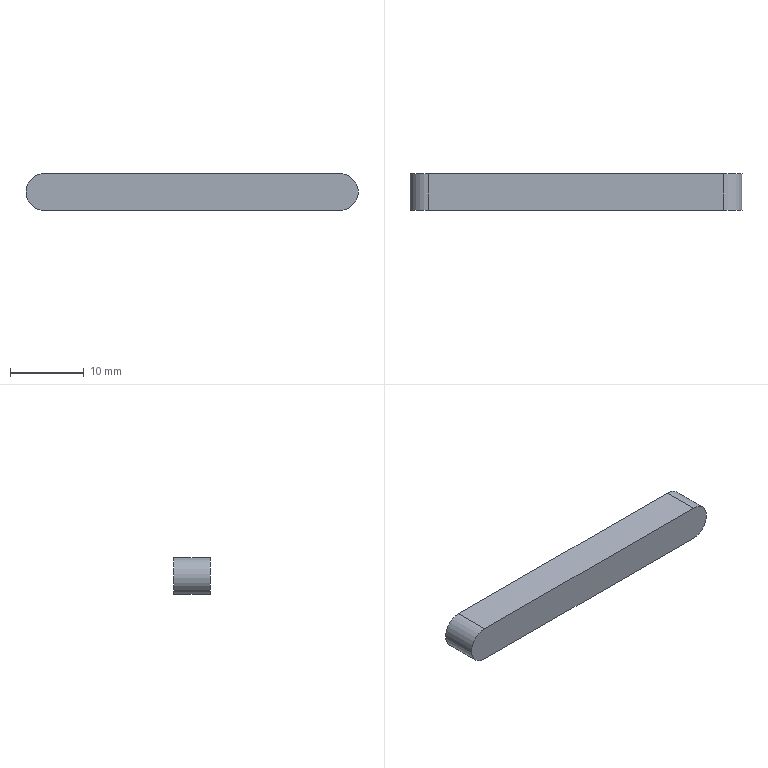Part | STEP file | PN_0046 (5x5x40) | 1 solid | 6 faces | box 45 x 5 x 5 mm | volume 1098 mm3 | plane 4 | cylinder 2 | commonest cylinder face diameters 5 x2
STEP:
#1=CARTESIAN_POINT('',(0.,0.,0.));
#2=DIRECTION('',(0.,0.,1.));
#3=DIRECTION('',(1.,0.,0.));
#4=AXIS2_PLACEMENT_3D('',#1,#2,#3);
#5=CARTESIAN_POINT('',(-20.,0.,-2.5));
#6=VERTEX_POINT('',#5);
#7=CARTESIAN_POINT('',(-20.,0.,2.5));
#8=VERTEX_POINT('',#7);
#9=CARTESIAN_POINT('',(-20.,0.,0.));
#10=DIRECTION('',(0.,1.,0.));
#11=DIRECTION('',(0.,0.,1.));
#12=AXIS2_PLACEMENT_3D('',#9,#10,#11);
#13=CIRCLE('',#12,2.5);
#14=CARTESIAN_POINT('',(-20.,5.,0.));
#15=DIRECTION('',(0.,-1.,0.));
#16=DIRECTION('',(0.,0.,-1.));
#17=AXIS2_PLACEMENT_3D('',#14,#15,#16);
#18=CYLINDRICAL_SURFACE('',#17,2.5);
#19=CARTESIAN_POINT('',(9.425,5.));
#20=DIRECTION('',(-1.,0.));
#21=VECTOR('',#20,1.);
#22=LINE('',#19,#21);
#23=(GEOMETRIC_REPRESENTATION_CONTEXT(2)PARAMETRIC_REPRESENTATION_CONTEXT()REPRESENTATION_CONTEXT('',''));
#24=DEFINITIONAL_REPRESENTATION('',(#22),#23);
#25=PCURVE('',#18,#24);
#26=CARTESIAN_POINT('',(-20.,0.,0.));
#27=DIRECTION('',(0.,1.,0.));
#28=DIRECTION('',(0.,0.,1.));
#29=AXIS2_PLACEMENT_3D('',#26,#27,#28);
#30=PLANE('',#29);
#31=CARTESIAN_POINT('',(0.,0.));
#32=DIRECTION('',(1.,0.));
#33=AXIS2_PLACEMENT_2D('',#31,#32);
#34=CIRCLE('',#33,2.5);
#35=(GEOMETRIC_REPRESENTATION_CONTEXT(2)PARAMETRIC_REPRESENTATION_CONTEXT()REPRESENTATION_CONTEXT('',''));
#36=DEFINITIONAL_REPRESENTATION('',(#34),#35);
#37=PCURVE('',#30,#36);
#38=SURFACE_CURVE('',#13,(#25,#37),.PCURVE_S1.);
#39=EDGE_CURVE('',#6,#8,#38,.T.);
#40=ORIENTED_EDGE('',*,*,#39,.T.);
#41=CARTESIAN_POINT('',(-20.,5.,2.5));
#42=VERTEX_POINT('',#41);
#43=CARTESIAN_POINT('',(-20.,5.,2.5));
#44=DIRECTION('',(0.,-1.,0.));
#45=VECTOR('',#44,1.);
#46=LINE('',#43,#45);
#47=CARTESIAN_POINT('',(3.142,0.));
#48=DIRECTION('',(0.,1.));
#49=VECTOR('',#48,1.);
#50=LINE('',#47,#49);
#51=(GEOMETRIC_REPRESENTATION_CONTEXT(2)PARAMETRIC_REPRESENTATION_CONTEXT()REPRESENTATION_CONTEXT('',''));
#52=DEFINITIONAL_REPRESENTATION('',(#50),#51);
#53=PCURVE('',#18,#52);
#54=CARTESIAN_POINT('',(-20.,5.,2.5));
#55=DIRECTION('',(0.,0.,-1.));
#56=DIRECTION('',(-1.,0.,0.));
#57=AXIS2_PLACEMENT_3D('',#54,#55,#56);
#58=PLANE('',#57);
#59=CARTESIAN_POINT('',(0.,0.));
#60=DIRECTION('',(0.,-1.));
#61=VECTOR('',#60,1.);
#62=LINE('',#59,#61);
#63=(GEOMETRIC_REPRESENTATION_CONTEXT(2)PARAMETRIC_REPRESENTATION_CONTEXT()REPRESENTATION_CONTEXT('',''));
#64=DEFINITIONAL_REPRESENTATION('',(#62),#63);
#65=PCURVE('',#58,#64);
#66=SURFACE_CURVE('',#46,(#53,#65),.PCURVE_S1.);
#67=EDGE_CURVE('',#42,#8,#66,.T.);
#68=ORIENTED_EDGE('',*,*,#67,.F.);
#69=CARTESIAN_POINT('',(-20.,5.,-2.5));
#70=VERTEX_POINT('',#69);
#71=CARTESIAN_POINT('',(-20.,5.,0.));
#72=DIRECTION('',(0.,1.,0.));
#73=DIRECTION('',(0.,0.,1.));
#74=AXIS2_PLACEMENT_3D('',#71,#72,#73);
#75=CIRCLE('',#74,2.5);
#76=CARTESIAN_POINT('',(9.425,0.));
#77=DIRECTION('',(-1.,0.));
#78=VECTOR('',#77,1.);
#79=LINE('',#76,#78);
#80=(GEOMETRIC_REPRESENTATION_CONTEXT(2)PARAMETRIC_REPRESENTATION_CONTEXT()REPRESENTATION_CONTEXT('',''));
#81=DEFINITIONAL_REPRESENTATION('',(#79),#80);
#82=PCURVE('',#18,#81);
#83=CARTESIAN_POINT('',(-20.,5.,0.));
#84=DIRECTION('',(0.,1.,0.));
#85=DIRECTION('',(0.,0.,1.));
#86=AXIS2_PLACEMENT_3D('',#83,#84,#85);
#87=PLANE('',#86);
#88=CARTESIAN_POINT('',(0.,0.));
#89=DIRECTION('',(1.,0.));
#90=AXIS2_PLACEMENT_2D('',#88,#89);
#91=CIRCLE('',#90,2.5);
#92=(GEOMETRIC_REPRESENTATION_CONTEXT(2)PARAMETRIC_REPRESENTATION_CONTEXT()REPRESENTATION_CONTEXT('',''));
#93=DEFINITIONAL_REPRESENTATION('',(#91),#92);
#94=PCURVE('',#87,#93);
#95=SURFACE_CURVE('',#75,(#82,#94),.PCURVE_S1.);
#96=EDGE_CURVE('',#70,#42,#95,.T.);
#97=ORIENTED_EDGE('',*,*,#96,.F.);
#98=CARTESIAN_POINT('',(-20.,5.,-2.5));
#99=DIRECTION('',(0.,-1.,0.));
#100=VECTOR('',#99,1.);
#101=LINE('',#98,#100);
#102=CARTESIAN_POINT('',(6.283,0.));
#103=DIRECTION('',(0.,1.));
#104=VECTOR('',#103,1.);
#105=LINE('',#102,#104);
#106=(GEOMETRIC_REPRESENTATION_CONTEXT(2)PARAMETRIC_REPRESENTATION_CONTEXT()REPRESENTATION_CONTEXT('',''));
#107=DEFINITIONAL_REPRESENTATION('',(#105),#106);
#108=PCURVE('',#18,#107);
#109=CARTESIAN_POINT('',(-20.,5.,-2.5));
#110=DIRECTION('',(0.,0.,1.));
#111=DIRECTION('',(1.,0.,0.));
#112=AXIS2_PLACEMENT_3D('',#109,#110,#111);
#113=PLANE('',#112);
#114=CARTESIAN_POINT('',(0.,0.));
#115=DIRECTION('',(0.,-1.));
#116=VECTOR('',#115,1.);
#117=LINE('',#114,#116);
#118=(GEOMETRIC_REPRESENTATION_CONTEXT(2)PARAMETRIC_REPRESENTATION_CONTEXT()REPRESENTATION_CONTEXT('',''));
#119=DEFINITIONAL_REPRESENTATION('',(#117),#118);
#120=PCURVE('',#113,#119);
#121=SURFACE_CURVE('',#101,(#108,#120),.PCURVE_S1.);
#122=EDGE_CURVE('',#70,#6,#121,.T.);
#123=ORIENTED_EDGE('',*,*,#122,.T.);
#124=EDGE_LOOP('',(#40,#68,#97,#123));
#125=FACE_BOUND('',#124,.T.);
#126=ADVANCED_FACE('',(#125),#18,.T.);
#127=CARTESIAN_POINT('',(20.,0.,2.5));
#128=VERTEX_POINT('',#127);
#129=CARTESIAN_POINT('',(-20.,0.,2.5));
#130=DIRECTION('',(1.,0.,0.));
#131=VECTOR('',#130,1.);
#132=LINE('',#129,#131);
#133=CARTESIAN_POINT('',(0.,-5.));
#134=DIRECTION('',(-1.,0.));
#135=VECTOR('',#134,1.);
#136=LINE('',#133,#135);
#137=(GEOMETRIC_REPRESENTATION_CONTEXT(2)PARAMETRIC_REPRESENTATION_CONTEXT()REPRESENTATION_CONTEXT('',''));
#138=DEFINITIONAL_REPRESENTATION('',(#136),#137);
#139=PCURVE('',#58,#138);
#140=CARTESIAN_POINT('',(2.5,0.));
#141=DIRECTION('',(0.,1.));
#142=VECTOR('',#141,1.);
#143=LINE('',#140,#142);
#144=(GEOMETRIC_REPRESENTATION_CONTEXT(2)PARAMETRIC_REPRESENTATION_CONTEXT()REPRESENTATION_CONTEXT('',''));
#145=DEFINITIONAL_REPRESENTATION('',(#143),#144);
#146=PCURVE('',#30,#145);
#147=SURFACE_CURVE('',#132,(#139,#146),.PCURVE_S1.);
#148=EDGE_CURVE('',#8,#128,#147,.T.);
#149=ORIENTED_EDGE('',*,*,#148,.T.);
#150=CARTESIAN_POINT('',(20.,5.,2.5));
#151=VERTEX_POINT('',#150);
#152=CARTESIAN_POINT('',(20.,5.,2.5));
#153=DIRECTION('',(0.,-1.,0.));
#154=VECTOR('',#153,1.);
#155=LINE('',#152,#154);
#156=CARTESIAN_POINT('',(-40.,0.));
#157=DIRECTION('',(0.,-1.));
#158=VECTOR('',#157,1.);
#159=LINE('',#156,#158);
#160=(GEOMETRIC_REPRESENTATION_CONTEXT(2)PARAMETRIC_REPRESENTATION_CONTEXT()REPRESENTATION_CONTEXT('',''));
#161=DEFINITIONAL_REPRESENTATION('',(#159),#160);
#162=PCURVE('',#58,#161);
#163=CARTESIAN_POINT('',(20.,5.,0.));
#164=DIRECTION('',(0.,-1.,0.));
#165=DIRECTION('',(0.,0.,-1.));
#166=AXIS2_PLACEMENT_3D('',#163,#164,#165);
#167=CYLINDRICAL_SURFACE('',#166,2.5);
#168=CARTESIAN_POINT('',(3.142,0.));
#169=DIRECTION('',(0.,1.));
#170=VECTOR('',#169,1.);
#171=LINE('',#168,#170);
#172=(GEOMETRIC_REPRESENTATION_CONTEXT(2)PARAMETRIC_REPRESENTATION_CONTEXT()REPRESENTATION_CONTEXT('',''));
#173=DEFINITIONAL_REPRESENTATION('',(#171),#172);
#174=PCURVE('',#167,#173);
#175=SURFACE_CURVE('',#155,(#162,#174),.PCURVE_S1.);
#176=EDGE_CURVE('',#151,#128,#175,.T.);
#177=ORIENTED_EDGE('',*,*,#176,.F.);
#178=CARTESIAN_POINT('',(-20.,5.,2.5));
#179=DIRECTION('',(1.,0.,0.));
#180=VECTOR('',#179,1.);
#181=LINE('',#178,#180);
#182=CARTESIAN_POINT('',(0.,0.));
#183=DIRECTION('',(-1.,0.));
#184=VECTOR('',#183,1.);
#185=LINE('',#182,#184);
#186=(GEOMETRIC_REPRESENTATION_CONTEXT(2)PARAMETRIC_REPRESENTATION_CONTEXT()REPRESENTATION_CONTEXT('',''));
#187=DEFINITIONAL_REPRESENTATION('',(#185),#186);
#188=PCURVE('',#58,#187);
#189=CARTESIAN_POINT('',(2.5,0.));
#190=DIRECTION('',(0.,1.));
#191=VECTOR('',#190,1.);
#192=LINE('',#189,#191);
#193=(GEOMETRIC_REPRESENTATION_CONTEXT(2)PARAMETRIC_REPRESENTATION_CONTEXT()REPRESENTATION_CONTEXT('',''));
#194=DEFINITIONAL_REPRESENTATION('',(#192),#193);
#195=PCURVE('',#87,#194);
#196=SURFACE_CURVE('',#181,(#188,#195),.PCURVE_S1.);
#197=EDGE_CURVE('',#42,#151,#196,.T.);
#198=ORIENTED_EDGE('',*,*,#197,.F.);
#199=ORIENTED_EDGE('',*,*,#67,.T.);
#200=EDGE_LOOP('',(#149,#177,#198,#199));
#201=FACE_BOUND('',#200,.T.);
#202=ADVANCED_FACE('',(#201),#58,.F.);
#203=CARTESIAN_POINT('',(20.,0.,-2.5));
#204=VERTEX_POINT('',#203);
#205=CARTESIAN_POINT('',(20.,0.,0.));
#206=DIRECTION('',(0.,1.,0.));
#207=DIRECTION('',(0.,0.,1.));
#208=AXIS2_PLACEMENT_3D('',#205,#206,#207);
#209=CIRCLE('',#208,2.5);
#210=CARTESIAN_POINT('',(3.142,5.));
#211=DIRECTION('',(-1.,0.));
#212=VECTOR('',#211,1.);
#213=LINE('',#210,#212);
#214=(GEOMETRIC_REPRESENTATION_CONTEXT(2)PARAMETRIC_REPRESENTATION_CONTEXT()REPRESENTATION_CONTEXT('',''));
#215=DEFINITIONAL_REPRESENTATION('',(#213),#214);
#216=PCURVE('',#167,#215);
#217=CARTESIAN_POINT('',(0.,40.));
#218=DIRECTION('',(1.,0.));
#219=AXIS2_PLACEMENT_2D('',#217,#218);
#220=CIRCLE('',#219,2.5);
#221=(GEOMETRIC_REPRESENTATION_CONTEXT(2)PARAMETRIC_REPRESENTATION_CONTEXT()REPRESENTATION_CONTEXT('',''));
#222=DEFINITIONAL_REPRESENTATION('',(#220),#221);
#223=PCURVE('',#30,#222);
#224=SURFACE_CURVE('',#209,(#216,#223),.PCURVE_S1.);
#225=EDGE_CURVE('',#128,#204,#224,.T.);
#226=ORIENTED_EDGE('',*,*,#225,.T.);
#227=CARTESIAN_POINT('',(20.,5.,-2.5));
#228=VERTEX_POINT('',#227);
#229=CARTESIAN_POINT('',(20.,5.,-2.5));
#230=DIRECTION('',(0.,-1.,0.));
#231=VECTOR('',#230,1.);
#232=LINE('',#229,#231);
#233=CARTESIAN_POINT('',(0.,0.));
#234=DIRECTION('',(0.,1.));
#235=VECTOR('',#234,1.);
#236=LINE('',#233,#235);
#237=(GEOMETRIC_REPRESENTATION_CONTEXT(2)PARAMETRIC_REPRESENTATION_CONTEXT()REPRESENTATION_CONTEXT('',''));
#238=DEFINITIONAL_REPRESENTATION('',(#236),#237);
#239=PCURVE('',#167,#238);
#240=CARTESIAN_POINT('',(40.,0.));
#241=DIRECTION('',(0.,-1.));
#242=VECTOR('',#241,1.);
#243=LINE('',#240,#242);
#244=(GEOMETRIC_REPRESENTATION_CONTEXT(2)PARAMETRIC_REPRESENTATION_CONTEXT()REPRESENTATION_CONTEXT('',''));
#245=DEFINITIONAL_REPRESENTATION('',(#243),#244);
#246=PCURVE('',#113,#245);
#247=SURFACE_CURVE('',#232,(#239,#246),.PCURVE_S1.);
#248=EDGE_CURVE('',#228,#204,#247,.T.);
#249=ORIENTED_EDGE('',*,*,#248,.F.);
#250=CARTESIAN_POINT('',(20.,5.,0.));
#251=DIRECTION('',(0.,1.,0.));
#252=DIRECTION('',(0.,0.,1.));
#253=AXIS2_PLACEMENT_3D('',#250,#251,#252);
#254=CIRCLE('',#253,2.5);
#255=CARTESIAN_POINT('',(3.142,0.));
#256=DIRECTION('',(-1.,0.));
#257=VECTOR('',#256,1.);
#258=LINE('',#255,#257);
#259=(GEOMETRIC_REPRESENTATION_CONTEXT(2)PARAMETRIC_REPRESENTATION_CONTEXT()REPRESENTATION_CONTEXT('',''));
#260=DEFINITIONAL_REPRESENTATION('',(#258),#259);
#261=PCURVE('',#167,#260);
#262=CARTESIAN_POINT('',(0.,40.));
#263=DIRECTION('',(1.,0.));
#264=AXIS2_PLACEMENT_2D('',#262,#263);
#265=CIRCLE('',#264,2.5);
#266=(GEOMETRIC_REPRESENTATION_CONTEXT(2)PARAMETRIC_REPRESENTATION_CONTEXT()REPRESENTATION_CONTEXT('',''));
#267=DEFINITIONAL_REPRESENTATION('',(#265),#266);
#268=PCURVE('',#87,#267);
#269=SURFACE_CURVE('',#254,(#261,#268),.PCURVE_S1.);
#270=EDGE_CURVE('',#151,#228,#269,.T.);
#271=ORIENTED_EDGE('',*,*,#270,.F.);
#272=ORIENTED_EDGE('',*,*,#176,.T.);
#273=EDGE_LOOP('',(#226,#249,#271,#272));
#274=FACE_BOUND('',#273,.T.);
#275=ADVANCED_FACE('',(#274),#167,.T.);
#276=CARTESIAN_POINT('',(-20.,0.,-2.5));
#277=DIRECTION('',(-1.,0.,0.));
#278=VECTOR('',#277,1.);
#279=LINE('',#276,#278);
#280=CARTESIAN_POINT('',(0.,-5.));
#281=DIRECTION('',(-1.,0.));
#282=VECTOR('',#281,1.);
#283=LINE('',#280,#282);
#284=(GEOMETRIC_REPRESENTATION_CONTEXT(2)PARAMETRIC_REPRESENTATION_CONTEXT()REPRESENTATION_CONTEXT('',''));
#285=DEFINITIONAL_REPRESENTATION('',(#283),#284);
#286=PCURVE('',#113,#285);
#287=CARTESIAN_POINT('',(-2.5,0.));
#288=DIRECTION('',(0.,-1.));
#289=VECTOR('',#288,1.);
#290=LINE('',#287,#289);
#291=(GEOMETRIC_REPRESENTATION_CONTEXT(2)PARAMETRIC_REPRESENTATION_CONTEXT()REPRESENTATION_CONTEXT('',''));
#292=DEFINITIONAL_REPRESENTATION('',(#290),#291);
#293=PCURVE('',#30,#292);
#294=SURFACE_CURVE('',#279,(#286,#293),.PCURVE_S1.);
#295=EDGE_CURVE('',#204,#6,#294,.T.);
#296=ORIENTED_EDGE('',*,*,#295,.T.);
#297=ORIENTED_EDGE('',*,*,#122,.F.);
#298=CARTESIAN_POINT('',(-20.,5.,-2.5));
#299=DIRECTION('',(-1.,0.,0.));
#300=VECTOR('',#299,1.);
#301=LINE('',#298,#300);
#302=CARTESIAN_POINT('',(0.,0.));
#303=DIRECTION('',(-1.,0.));
#304=VECTOR('',#303,1.);
#305=LINE('',#302,#304);
#306=(GEOMETRIC_REPRESENTATION_CONTEXT(2)PARAMETRIC_REPRESENTATION_CONTEXT()REPRESENTATION_CONTEXT('',''));
#307=DEFINITIONAL_REPRESENTATION('',(#305),#306);
#308=PCURVE('',#113,#307);
#309=CARTESIAN_POINT('',(-2.5,0.));
#310=DIRECTION('',(0.,-1.));
#311=VECTOR('',#310,1.);
#312=LINE('',#309,#311);
#313=(GEOMETRIC_REPRESENTATION_CONTEXT(2)PARAMETRIC_REPRESENTATION_CONTEXT()REPRESENTATION_CONTEXT('',''));
#314=DEFINITIONAL_REPRESENTATION('',(#312),#313);
#315=PCURVE('',#87,#314);
#316=SURFACE_CURVE('',#301,(#308,#315),.PCURVE_S1.);
#317=EDGE_CURVE('',#228,#70,#316,.T.);
#318=ORIENTED_EDGE('',*,*,#317,.F.);
#319=ORIENTED_EDGE('',*,*,#248,.T.);
#320=EDGE_LOOP('',(#296,#297,#318,#319));
#321=FACE_BOUND('',#320,.T.);
#322=ADVANCED_FACE('',(#321),#113,.F.);
#323=ORIENTED_EDGE('',*,*,#96,.T.);
#324=ORIENTED_EDGE('',*,*,#197,.T.);
#325=ORIENTED_EDGE('',*,*,#270,.T.);
#326=ORIENTED_EDGE('',*,*,#317,.T.);
#327=EDGE_LOOP('',(#323,#324,#325,#326));
#328=FACE_BOUND('',#327,.T.);
#329=ADVANCED_FACE('',(#328),#87,.T.);
#330=ORIENTED_EDGE('',*,*,#39,.F.);
#331=ORIENTED_EDGE('',*,*,#295,.F.);
#332=ORIENTED_EDGE('',*,*,#225,.F.);
#333=ORIENTED_EDGE('',*,*,#148,.F.);
#334=EDGE_LOOP('',(#330,#331,#332,#333));
#335=FACE_BOUND('',#334,.T.);
#336=ADVANCED_FACE('',(#335),#30,.F.);
#337=CLOSED_SHELL('',(#126,#202,#275,#322,#329,#336));
#338=MANIFOLD_SOLID_BREP('',#337);
#339=(LENGTH_UNIT()NAMED_UNIT(*)SI_UNIT(.MILLI.,.METRE.));
#340=UNCERTAINTY_MEASURE_WITH_UNIT(LENGTH_MEASURE(0.0000001),#339,'','');
#341=(NAMED_UNIT(*)PLANE_ANGLE_UNIT()SI_UNIT($,.RADIAN.));
#342=(NAMED_UNIT(*)SI_UNIT($,.STERADIAN.)SOLID_ANGLE_UNIT());
#343=(GEOMETRIC_REPRESENTATION_CONTEXT(3)GLOBAL_UNCERTAINTY_ASSIGNED_CONTEXT((#340))GLOBAL_UNIT_ASSIGNED_CONTEXT((#339,#341,#342))REPRESENTATION_CONTEXT('',''));
#344=ADVANCED_BREP_SHAPE_REPRESENTATION('',(#4,#338),#343);